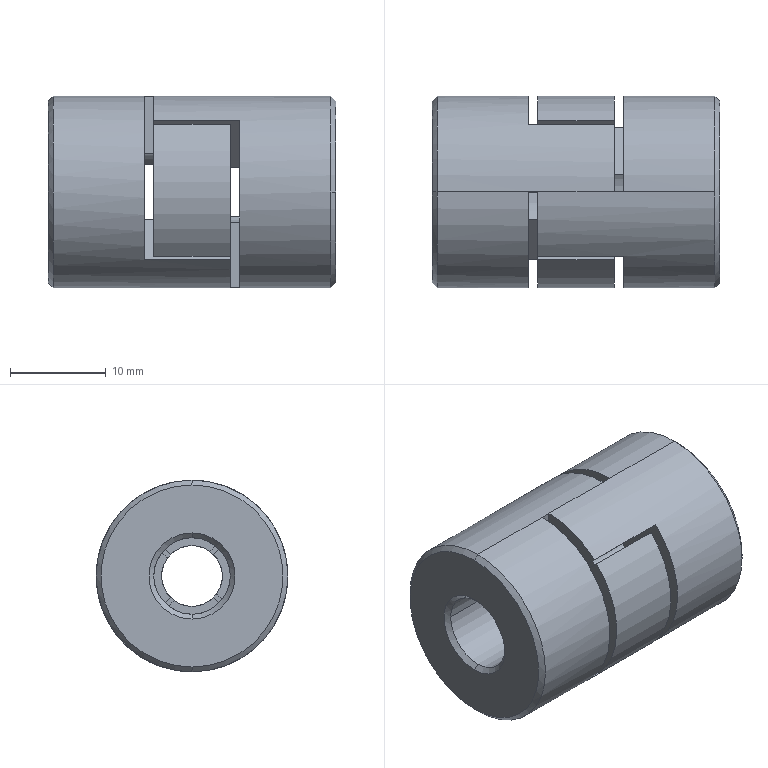Part | STEP file | Coupling CPJC 20 RD φ6.35-φ8 | 3 solids | 55 faces | box 30 x 20 x 20 mm | volume 7655 mm3 | plane 30 | cylinder 17 | cone 8 | commonest cylinder face diameters 6.35 x6 20 x6 8 x5